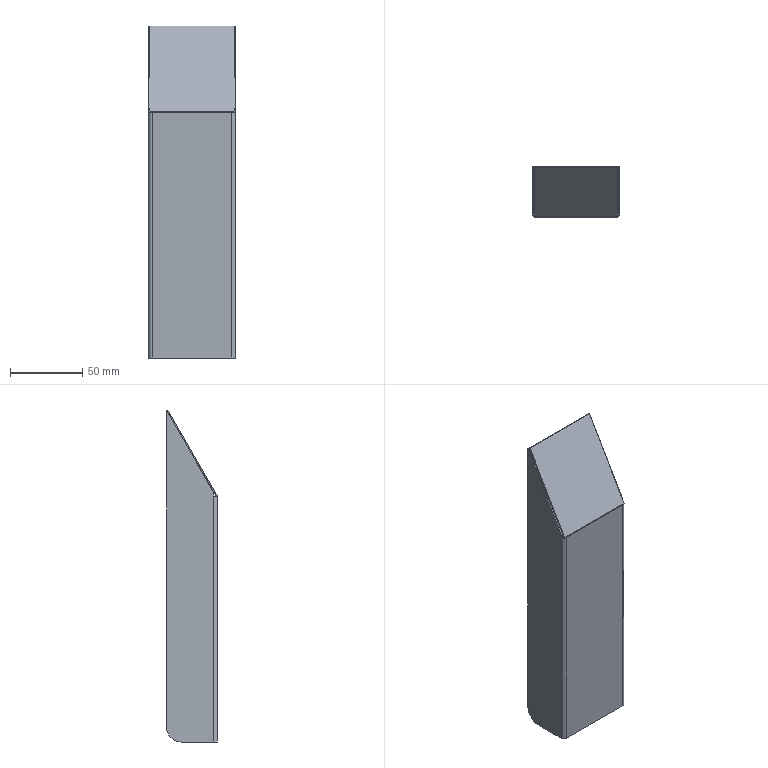Part | NX | 1 solid | 36 faces | box 60 x 35 x 229.016 mm | volume 27274 mm3 | plane 24 | cylinder 12 | commonest cylinder face diameters 4.5 x4 3.2 x2 5.2 x2 20 x2 0.8 x1 2.8 x1
STEP:
#1=CARTESIAN_POINT('',(2020.571,-112.446,-328.341));
#2=VERTEX_POINT('',#1);
#3=CARTESIAN_POINT('',(2020.571,-113.312,-327.841));
#4=VERTEX_POINT('',#3);
#5=CARTESIAN_POINT('',(2020.571,-112.446,-328.341));
#6=DIRECTION('',(0.,-0.866,0.5));
#7=VECTOR('',#6,1000.);
#8=LINE('',#5,#7);
#9=EDGE_CURVE('',#2,#4,#8,.T.);
#10=ORIENTED_EDGE('',*,*,#9,.T.);
#11=CARTESIAN_POINT('',(2020.571,-79.427,-269.151));
#12=VERTEX_POINT('',#11);
#13=CARTESIAN_POINT('',(2020.571,-171.235,-428.166));
#14=DIRECTION('',(0.,0.5,0.866));
#15=VECTOR('',#14,1000.);
#16=LINE('',#13,#15);
#17=EDGE_CURVE('',#4,#12,#16,.T.);
#18=ORIENTED_EDGE('',*,*,#17,.T.);
#19=CARTESIAN_POINT('',(2020.571,-78.561,-269.651));
#20=VERTEX_POINT('',#19);
#21=CARTESIAN_POINT('',(2020.571,-112.5,-250.056));
#22=DIRECTION('',(0.,0.866,-0.5));
#23=VECTOR('',#22,1000.);
#24=LINE('',#21,#23);
#25=EDGE_CURVE('',#12,#20,#24,.T.);
#26=ORIENTED_EDGE('',*,*,#25,.T.);
#27=CARTESIAN_POINT('',(2020.571,-170.08,-428.166));
#28=DIRECTION('',(0.,0.5,0.866));
#29=VECTOR('',#28,1000.);
#30=LINE('',#27,#29);
#31=EDGE_CURVE('',#2,#20,#30,.T.);
#32=ORIENTED_EDGE('',*,*,#31,.F.);
#33=EDGE_LOOP('',(#10,#18,#26,#32));
#34=FACE_BOUND('',#33,.T.);
#35=CARTESIAN_POINT('',(2020.571,-103.79,-313.348));
#36=DIRECTION('',(-1.,0.,0.));
#37=DIRECTION('',(0.,0.,1.));
#38=AXIS2_PLACEMENT_3D('',#35,#36,#37);
#39=PLANE('',#38);
#40=ADVANCED_FACE('',(#34),#39,.T.);
#41=CARTESIAN_POINT('',(2020.5,-88.5,-498.166));
#42=VERTEX_POINT('',#41);
#43=CARTESIAN_POINT('',(2019.5,-88.5,-498.166));
#44=VERTEX_POINT('',#43);
#45=CARTESIAN_POINT('',(1649.5,-88.5,-498.166));
#46=DIRECTION('',(-1.,0.,0.));
#47=VECTOR('',#46,1000.);
#48=LINE('',#45,#47);
#49=EDGE_CURVE('',#42,#44,#48,.T.);
#50=ORIENTED_EDGE('',*,*,#49,.F.);
#51=CARTESIAN_POINT('',(2020.5,-110.9,-498.166));
#52=VERTEX_POINT('',#51);
#53=CARTESIAN_POINT('',(2020.5,-112.5,-498.166));
#54=DIRECTION('',(0.,-1.,0.));
#55=VECTOR('',#54,1000.);
#56=LINE('',#53,#55);
#57=EDGE_CURVE('',#42,#52,#56,.T.);
#58=ORIENTED_EDGE('',*,*,#57,.T.);
#59=CARTESIAN_POINT('',(2022.1,-112.5,-498.166));
#60=VERTEX_POINT('',#59);
#61=CARTESIAN_POINT('',(2022.1,-110.9,-498.166));
#62=DIRECTION('',(0.,0.,1.));
#63=DIRECTION('',(-1.,0.,0.));
#64=AXIS2_PLACEMENT_3D('',#61,#62,#63);
#65=CIRCLE('',#64,1.6);
#66=EDGE_CURVE('',#52,#60,#65,.T.);
#67=ORIENTED_EDGE('',*,*,#66,.T.);
#68=CARTESIAN_POINT('',(2076.9,-112.5,-498.166));
#69=VERTEX_POINT('',#68);
#70=CARTESIAN_POINT('',(1649.5,-112.5,-498.166));
#71=DIRECTION('',(1.,0.,0.));
#72=VECTOR('',#71,1000.);
#73=LINE('',#70,#72);
#74=EDGE_CURVE('',#60,#69,#73,.T.);
#75=ORIENTED_EDGE('',*,*,#74,.T.);
#76=CARTESIAN_POINT('',(2078.5,-110.9,-498.166));
#77=VERTEX_POINT('',#76);
#78=CARTESIAN_POINT('',(2076.9,-110.9,-498.166));
#79=DIRECTION('',(0.,0.,-1.));
#80=DIRECTION('',(1.,0.,0.));
#81=AXIS2_PLACEMENT_3D('',#78,#79,#80);
#82=CIRCLE('',#81,1.6);
#83=EDGE_CURVE('',#77,#69,#82,.T.);
#84=ORIENTED_EDGE('',*,*,#83,.F.);
#85=CARTESIAN_POINT('',(2078.5,-88.5,-498.166));
#86=VERTEX_POINT('',#85);
#87=CARTESIAN_POINT('',(2078.5,-112.5,-498.166));
#88=DIRECTION('',(0.,1.,0.));
#89=VECTOR('',#88,1000.);
#90=LINE('',#87,#89);
#91=EDGE_CURVE('',#77,#86,#90,.T.);
#92=ORIENTED_EDGE('',*,*,#91,.T.);
#93=CARTESIAN_POINT('',(2079.5,-88.5,-498.166));
#94=VERTEX_POINT('',#93);
#95=CARTESIAN_POINT('',(1649.5,-88.5,-498.166));
#96=DIRECTION('',(-1.,0.,0.));
#97=VECTOR('',#96,1000.);
#98=LINE('',#95,#97);
#99=EDGE_CURVE('',#94,#86,#98,.T.);
#100=ORIENTED_EDGE('',*,*,#99,.F.);
#101=CARTESIAN_POINT('',(2079.5,-110.9,-498.166));
#102=VERTEX_POINT('',#101);
#103=CARTESIAN_POINT('',(2079.5,-112.5,-498.166));
#104=DIRECTION('',(0.,-1.,0.));
#105=VECTOR('',#104,1000.);
#106=LINE('',#103,#105);
#107=EDGE_CURVE('',#94,#102,#106,.T.);
#108=ORIENTED_EDGE('',*,*,#107,.T.);
#109=CARTESIAN_POINT('',(2076.9,-113.5,-498.166));
#110=VERTEX_POINT('',#109);
#111=CARTESIAN_POINT('',(2076.9,-110.9,-498.166));
#112=DIRECTION('',(0.,0.,-1.));
#113=DIRECTION('',(1.,0.,0.));
#114=AXIS2_PLACEMENT_3D('',#111,#112,#113);
#115=CIRCLE('',#114,2.6);
#116=EDGE_CURVE('',#102,#110,#115,.T.);
#117=ORIENTED_EDGE('',*,*,#116,.T.);
#118=CARTESIAN_POINT('',(2022.1,-113.5,-498.166));
#119=VERTEX_POINT('',#118);
#120=CARTESIAN_POINT('',(1649.5,-113.5,-498.166));
#121=DIRECTION('',(1.,0.,0.));
#122=VECTOR('',#121,1000.);
#123=LINE('',#120,#122);
#124=EDGE_CURVE('',#119,#110,#123,.T.);
#125=ORIENTED_EDGE('',*,*,#124,.F.);
#126=CARTESIAN_POINT('',(2019.5,-110.9,-498.166));
#127=VERTEX_POINT('',#126);
#128=CARTESIAN_POINT('',(2022.1,-110.9,-498.166));
#129=DIRECTION('',(0.,0.,1.));
#130=DIRECTION('',(-1.,0.,0.));
#131=AXIS2_PLACEMENT_3D('',#128,#129,#130);
#132=CIRCLE('',#131,2.6);
#133=EDGE_CURVE('',#127,#119,#132,.T.);
#134=ORIENTED_EDGE('',*,*,#133,.F.);
#135=CARTESIAN_POINT('',(2019.5,-112.5,-498.166));
#136=DIRECTION('',(0.,-1.,0.));
#137=VECTOR('',#136,1000.);
#138=LINE('',#135,#137);
#139=EDGE_CURVE('',#44,#127,#138,.T.);
#140=ORIENTED_EDGE('',*,*,#139,.F.);
#141=EDGE_LOOP('',(#50,#58,#67,#75,#84,#92,#100,#108,#117,#125,#134,#140));
#142=FACE_BOUND('',#141,.T.);
#143=CARTESIAN_POINT('',(2021.6,-170.4,-498.166));
#144=DIRECTION('',(0.,0.,-1.));
#145=DIRECTION('',(0.,-1.,0.));
#146=AXIS2_PLACEMENT_3D('',#143,#144,#145);
#147=PLANE('',#146);
#148=ADVANCED_FACE('',(#142),#147,.T.);
#149=CARTESIAN_POINT('',(2078.429,-113.312,-327.841));
#150=VERTEX_POINT('',#149);
#151=CARTESIAN_POINT('',(2078.429,-112.446,-328.341));
#152=VERTEX_POINT('',#151);
#153=CARTESIAN_POINT('',(2078.429,-112.446,-328.341));
#154=DIRECTION('',(0.,0.866,-0.5));
#155=VECTOR('',#154,1000.);
#156=LINE('',#153,#155);
#157=EDGE_CURVE('',#150,#152,#156,.T.);
#158=ORIENTED_EDGE('',*,*,#157,.T.);
#159=CARTESIAN_POINT('',(2078.429,-78.561,-269.651));
#160=VERTEX_POINT('',#159);
#161=CARTESIAN_POINT('',(2078.429,-170.08,-428.166));
#162=DIRECTION('',(0.,-0.5,-0.866));
#163=VECTOR('',#162,1000.);
#164=LINE('',#161,#163);
#165=EDGE_CURVE('',#160,#152,#164,.T.);
#166=ORIENTED_EDGE('',*,*,#165,.F.);
#167=CARTESIAN_POINT('',(2078.429,-79.427,-269.151));
#168=VERTEX_POINT('',#167);
#169=CARTESIAN_POINT('',(2078.429,-112.5,-250.056));
#170=DIRECTION('',(0.,-0.866,0.5));
#171=VECTOR('',#170,1000.);
#172=LINE('',#169,#171);
#173=EDGE_CURVE('',#160,#168,#172,.T.);
#174=ORIENTED_EDGE('',*,*,#173,.T.);
#175=CARTESIAN_POINT('',(2078.429,-171.235,-428.166));
#176=DIRECTION('',(0.,-0.5,-0.866));
#177=VECTOR('',#176,1000.);
#178=LINE('',#175,#177);
#179=EDGE_CURVE('',#168,#150,#178,.T.);
#180=ORIENTED_EDGE('',*,*,#179,.T.);
#181=EDGE_LOOP('',(#158,#166,#174,#180));
#182=FACE_BOUND('',#181,.T.);
#183=CARTESIAN_POINT('',(2078.429,-103.79,-313.348));
#184=DIRECTION('',(1.,0.,0.));
#185=DIRECTION('',(0.,1.,0.));
#186=AXIS2_PLACEMENT_3D('',#183,#184,#185);
#187=PLANE('',#186);
#188=ADVANCED_FACE('',(#182),#187,.T.);
#189=ORIENTED_EDGE('',*,*,#49,.T.);
#190=CARTESIAN_POINT('',(2019.5,-78.5,-488.166));
#191=VERTEX_POINT('',#190);
#192=CARTESIAN_POINT('',(2019.5,-88.5,-488.166));
#193=DIRECTION('',(-1.,0.,0.));
#194=DIRECTION('',(0.,0.,-1.));
#195=AXIS2_PLACEMENT_3D('',#192,#193,#194);
#196=CIRCLE('',#195,10.);
#197=EDGE_CURVE('',#191,#44,#196,.T.);
#198=ORIENTED_EDGE('',*,*,#197,.F.);
#199=CARTESIAN_POINT('',(2020.5,-78.5,-488.166));
#200=VERTEX_POINT('',#199);
#201=CARTESIAN_POINT('',(1649.5,-78.5,-488.166));
#202=DIRECTION('',(-1.,0.,0.));
#203=VECTOR('',#202,1000.);
#204=LINE('',#201,#203);
#205=EDGE_CURVE('',#200,#191,#204,.T.);
#206=ORIENTED_EDGE('',*,*,#205,.F.);
#207=CARTESIAN_POINT('',(2020.5,-88.5,-488.166));
#208=DIRECTION('',(-1.,0.,0.));
#209=DIRECTION('',(0.,0.,-1.));
#210=AXIS2_PLACEMENT_3D('',#207,#208,#209);
#211=CIRCLE('',#210,10.);
#212=EDGE_CURVE('',#200,#42,#211,.T.);
#213=ORIENTED_EDGE('',*,*,#212,.T.);
#214=EDGE_LOOP('',(#189,#198,#206,#213));
#215=FACE_BOUND('',#214,.T.);
#216=CARTESIAN_POINT('',(1649.5,-88.5,-488.166));
#217=DIRECTION('',(-1.,0.,0.));
#218=DIRECTION('',(0.,0.,-1.));
#219=AXIS2_PLACEMENT_3D('',#216,#217,#218);
#220=CYLINDRICAL_SURFACE('',#219,10.);
#221=ADVANCED_FACE('',(#215),#220,.T.);
#222=CARTESIAN_POINT('',(2079.5,-110.9,-328.541));
#223=VERTEX_POINT('',#222);
#224=CARTESIAN_POINT('',(2079.5,-110.9,-448.166));
#225=DIRECTION('',(0.,0.,-1.));
#226=VECTOR('',#225,1000.);
#227=LINE('',#224,#226);
#228=EDGE_CURVE('',#223,#102,#227,.T.);
#229=ORIENTED_EDGE('',*,*,#228,.T.);
#230=ORIENTED_EDGE('',*,*,#107,.F.);
#231=CARTESIAN_POINT('',(2079.5,-78.5,-488.166));
#232=VERTEX_POINT('',#231);
#233=CARTESIAN_POINT('',(2079.5,-88.5,-488.166));
#234=DIRECTION('',(-1.,0.,0.));
#235=DIRECTION('',(0.,0.,-1.));
#236=AXIS2_PLACEMENT_3D('',#233,#234,#235);
#237=CIRCLE('',#236,10.);
#238=EDGE_CURVE('',#232,#94,#237,.T.);
#239=ORIENTED_EDGE('',*,*,#238,.F.);
#240=CARTESIAN_POINT('',(2079.5,-78.5,-269.686));
#241=VERTEX_POINT('',#240);
#242=CARTESIAN_POINT('',(2079.5,-78.5,-428.166));
#243=DIRECTION('',(0.,0.,-1.));
#244=VECTOR('',#243,1000.);
#245=LINE('',#242,#244);
#246=EDGE_CURVE('',#241,#232,#245,.T.);
#247=ORIENTED_EDGE('',*,*,#246,.F.);
#248=CARTESIAN_POINT('',(2079.5,-110.9,-325.804));
#249=VERTEX_POINT('',#248);
#250=CARTESIAN_POINT('',(2079.5,-169.999,-428.166));
#251=DIRECTION('',(0.,0.5,0.866));
#252=VECTOR('',#251,1000.);
#253=LINE('',#250,#252);
#254=EDGE_CURVE('',#249,#241,#253,.T.);
#255=ORIENTED_EDGE('',*,*,#254,.F.);
#256=CARTESIAN_POINT('',(2079.5,-110.9,-428.166));
#257=DIRECTION('',(0.,0.,1.));
#258=VECTOR('',#257,1000.);
#259=LINE('',#256,#258);
#260=EDGE_CURVE('',#223,#249,#259,.T.);
#261=ORIENTED_EDGE('',*,*,#260,.F.);
#262=EDGE_LOOP('',(#229,#230,#239,#247,#255,#261));
#263=FACE_BOUND('',#262,.T.);
#264=CARTESIAN_POINT('',(2079.5,-86.551,-317.041));
#265=VERTEX_POINT('',#264);
#266=CARTESIAN_POINT('',(2079.5,-90.449,-319.291));
#267=VERTEX_POINT('',#266);
#268=CARTESIAN_POINT('',(2079.5,-88.5,-318.166));
#269=DIRECTION('',(-1.,0.,0.));
#270=DIRECTION('',(0.,-0.866,-0.5));
#271=AXIS2_PLACEMENT_3D('',#268,#269,#270);
#272=CIRCLE('',#271,2.25);
#273=EDGE_CURVE('',#265,#267,#272,.T.);
#274=ORIENTED_EDGE('',*,*,#273,.T.);
#275=CARTESIAN_POINT('',(2079.5,-88.5,-318.166));
#276=DIRECTION('',(-1.,0.,0.));
#277=DIRECTION('',(0.,-0.866,-0.5));
#278=AXIS2_PLACEMENT_3D('',#275,#276,#277);
#279=CIRCLE('',#278,2.25);
#280=EDGE_CURVE('',#267,#265,#279,.T.);
#281=ORIENTED_EDGE('',*,*,#280,.T.);
#282=EDGE_LOOP('',(#274,#281));
#283=FACE_BOUND('',#282,.T.);
#284=CARTESIAN_POINT('',(2079.5,-90.449,-364.291));
#285=VERTEX_POINT('',#284);
#286=CARTESIAN_POINT('',(2079.5,-86.551,-362.041));
#287=VERTEX_POINT('',#286);
#288=CARTESIAN_POINT('',(2079.5,-88.5,-363.166));
#289=DIRECTION('',(-1.,0.,0.));
#290=DIRECTION('',(0.,-0.866,-0.5));
#291=AXIS2_PLACEMENT_3D('',#288,#289,#290);
#292=CIRCLE('',#291,2.25);
#293=EDGE_CURVE('',#285,#287,#292,.T.);
#294=ORIENTED_EDGE('',*,*,#293,.T.);
#295=CARTESIAN_POINT('',(2079.5,-88.5,-363.166));
#296=DIRECTION('',(-1.,0.,0.));
#297=DIRECTION('',(0.,-0.866,-0.5));
#298=AXIS2_PLACEMENT_3D('',#295,#296,#297);
#299=CIRCLE('',#298,2.25);
#300=EDGE_CURVE('',#287,#285,#299,.T.);
#301=ORIENTED_EDGE('',*,*,#300,.T.);
#302=EDGE_LOOP('',(#294,#301));
#303=FACE_BOUND('',#302,.T.);
#304=CARTESIAN_POINT('',(2079.5,-541.4,-428.166));
#305=DIRECTION('',(-1.,0.,0.));
#306=DIRECTION('',(0.,0.,1.));
#307=AXIS2_PLACEMENT_3D('',#304,#305,#306);
#308=PLANE('',#307);
#309=ADVANCED_FACE('',(#263,#283,#303),#308,.F.);
#310=CARTESIAN_POINT('',(2022.1,-113.312,-327.841));
#311=VERTEX_POINT('',#310);
#312=CARTESIAN_POINT('',(2022.1,-113.5,-328.541));
#313=VERTEX_POINT('',#312);
#314=CARTESIAN_POINT('',(2022.1,-112.1,-328.541));
#315=DIRECTION('',(1.,0.,0.));
#316=DIRECTION('',(0.,-0.866,0.5));
#317=AXIS2_PLACEMENT_3D('',#314,#315,#316);
#318=CIRCLE('',#317,1.4);
#319=EDGE_CURVE('',#311,#313,#318,.T.);
#320=ORIENTED_EDGE('',*,*,#319,.T.);
#321=CARTESIAN_POINT('',(2076.9,-113.5,-328.541));
#322=VERTEX_POINT('',#321);
#323=CARTESIAN_POINT('',(1649.5,-113.5,-328.541));
#324=DIRECTION('',(-1.,0.,0.));
#325=VECTOR('',#324,1000.);
#326=LINE('',#323,#325);
#327=EDGE_CURVE('',#322,#313,#326,.T.);
#328=ORIENTED_EDGE('',*,*,#327,.F.);
#329=CARTESIAN_POINT('',(2076.9,-113.312,-327.841));
#330=VERTEX_POINT('',#329);
#331=CARTESIAN_POINT('',(2076.9,-112.1,-328.541));
#332=DIRECTION('',(-1.,0.,0.));
#333=DIRECTION('',(0.,-1.,0.));
#334=AXIS2_PLACEMENT_3D('',#331,#332,#333);
#335=CIRCLE('',#334,1.4);
#336=EDGE_CURVE('',#322,#330,#335,.T.);
#337=ORIENTED_EDGE('',*,*,#336,.T.);
#338=CARTESIAN_POINT('',(1649.5,-113.312,-327.841));
#339=DIRECTION('',(-1.,0.,0.));
#340=VECTOR('',#339,1000.);
#341=LINE('',#338,#340);
#342=EDGE_CURVE('',#330,#311,#341,.T.);
#343=ORIENTED_EDGE('',*,*,#342,.T.);
#344=EDGE_LOOP('',(#320,#328,#337,#343));
#345=FACE_BOUND('',#344,.T.);
#346=CARTESIAN_POINT('',(2076.9,-112.1,-328.541));
#347=DIRECTION('',(1.,0.,0.));
#348=DIRECTION('',(0.,0.,1.));
#349=AXIS2_PLACEMENT_3D('',#346,#347,#348);
#350=CYLINDRICAL_SURFACE('',#349,1.4);
#351=ADVANCED_FACE('',(#345),#350,.T.);
#352=CARTESIAN_POINT('',(1649.5,-113.312,-327.841));
#353=DIRECTION('',(1.,0.,0.));
#354=VECTOR('',#353,1000.);
#355=LINE('',#352,#354);
#356=EDGE_CURVE('',#4,#311,#355,.T.);
#357=ORIENTED_EDGE('',*,*,#356,.T.);
#358=ORIENTED_EDGE('',*,*,#342,.F.);
#359=CARTESIAN_POINT('',(1649.5,-113.312,-327.841));
#360=DIRECTION('',(1.,0.,0.));
#361=VECTOR('',#360,1000.);
#362=LINE('',#359,#361);
#363=EDGE_CURVE('',#330,#150,#362,.T.);
#364=ORIENTED_EDGE('',*,*,#363,.T.);
#365=ORIENTED_EDGE('',*,*,#179,.F.);
#366=CARTESIAN_POINT('',(1649.5,-79.427,-269.151));
#367=DIRECTION('',(1.,0.,0.));
#368=VECTOR('',#367,1000.);
#369=LINE('',#366,#368);
#370=EDGE_CURVE('',#12,#168,#369,.T.);
#371=ORIENTED_EDGE('',*,*,#370,.F.);
#372=ORIENTED_EDGE('',*,*,#17,.F.);
#373=EDGE_LOOP('',(#357,#358,#364,#365,#371,#372));
#374=FACE_BOUND('',#373,.T.);
#375=CARTESIAN_POINT('',(1649.5,-163.289,-414.403));
#376=DIRECTION('',(0.,0.866,-0.5));
#377=DIRECTION('',(-1.,0.,0.));
#378=AXIS2_PLACEMENT_3D('',#375,#376,#377);
#379=PLANE('',#378);
#380=ADVANCED_FACE('',(#374),#379,.F.);
#381=CARTESIAN_POINT('',(2076.9,-113.5,-428.166));
#382=DIRECTION('',(0.,0.,1.));
#383=VECTOR('',#382,1000.);
#384=LINE('',#381,#383);
#385=EDGE_CURVE('',#110,#322,#384,.T.);
#386=ORIENTED_EDGE('',*,*,#385,.F.);
#387=ORIENTED_EDGE('',*,*,#116,.F.);
#388=ORIENTED_EDGE('',*,*,#228,.F.);
#389=CARTESIAN_POINT('',(2076.9,-110.9,-328.541));
#390=DIRECTION('',(0.,0.,-1.));
#391=DIRECTION('',(1.,0.,0.));
#392=AXIS2_PLACEMENT_3D('',#389,#390,#391);
#393=CIRCLE('',#392,2.6);
#394=EDGE_CURVE('',#223,#322,#393,.T.);
#395=ORIENTED_EDGE('',*,*,#394,.T.);
#396=EDGE_LOOP('',(#386,#387,#388,#395));
#397=FACE_BOUND('',#396,.T.);
#398=CARTESIAN_POINT('',(2076.9,-110.9,-448.166));
#399=DIRECTION('',(0.,0.,-1.));
#400=DIRECTION('',(1.,0.,0.));
#401=AXIS2_PLACEMENT_3D('',#398,#399,#400);
#402=CYLINDRICAL_SURFACE('',#401,2.6);
#403=ADVANCED_FACE('',(#397),#402,.T.);
#404=CARTESIAN_POINT('',(2078.5,-86.551,-362.041));
#405=VERTEX_POINT('',#404);
#406=CARTESIAN_POINT('',(2078.5,-90.449,-364.291));
#407=VERTEX_POINT('',#406);
#408=CARTESIAN_POINT('',(2078.5,-88.5,-363.166));
#409=DIRECTION('',(-1.,0.,0.));
#410=DIRECTION('',(0.,-0.866,-0.5));
#411=AXIS2_PLACEMENT_3D('',#408,#409,#410);
#412=CIRCLE('',#411,2.25);
#413=EDGE_CURVE('',#405,#407,#412,.T.);
#414=ORIENTED_EDGE('',*,*,#413,.T.);
#415=CARTESIAN_POINT('',(2085.5,-90.449,-364.291));
#416=DIRECTION('',(-1.,0.,0.));
#417=VECTOR('',#416,1000.);
#418=LINE('',#415,#417);
#419=EDGE_CURVE('',#407,#285,#418,.F.);
#420=ORIENTED_EDGE('',*,*,#419,.T.);
#421=ORIENTED_EDGE('',*,*,#300,.F.);
#422=CARTESIAN_POINT('',(2085.5,-86.551,-362.041));
#423=DIRECTION('',(-1.,0.,0.));
#424=VECTOR('',#423,1000.);
#425=LINE('',#422,#424);
#426=EDGE_CURVE('',#405,#287,#425,.F.);
#427=ORIENTED_EDGE('',*,*,#426,.F.);
#428=EDGE_LOOP('',(#414,#420,#421,#427));
#429=FACE_BOUND('',#428,.T.);
#430=CARTESIAN_POINT('',(2085.5,-88.5,-363.166));
#431=DIRECTION('',(-1.,0.,0.));
#432=DIRECTION('',(0.,-0.866,-0.5));
#433=AXIS2_PLACEMENT_3D('',#430,#431,#432);
#434=CYLINDRICAL_SURFACE('',#433,2.25);
#435=ADVANCED_FACE('',(#429),#434,.F.);
#436=ORIENTED_EDGE('',*,*,#356,.F.);
#437=ORIENTED_EDGE('',*,*,#9,.F.);
#438=CARTESIAN_POINT('',(2022.1,-112.446,-328.341));
#439=VERTEX_POINT('',#438);
#440=CARTESIAN_POINT('',(1649.5,-112.446,-328.341));
#441=DIRECTION('',(-1.,0.,0.));
#442=VECTOR('',#441,1000.);
#443=LINE('',#440,#442);
#444=EDGE_CURVE('',#439,#2,#443,.T.);
#445=ORIENTED_EDGE('',*,*,#444,.F.);
#446=CARTESIAN_POINT('',(2022.1,-113.312,-327.841));
#447=DIRECTION('',(0.,0.866,-0.5));
#448=VECTOR('',#447,1000.);
#449=LINE('',#446,#448);
#450=EDGE_CURVE('',#311,#439,#449,.T.);
#451=ORIENTED_EDGE('',*,*,#450,.F.);
#452=EDGE_LOOP('',(#436,#437,#445,#451));
#453=FACE_BOUND('',#452,.T.);
#454=CARTESIAN_POINT('',(2019.,-113.312,-327.841));
#455=DIRECTION('',(0.,-0.5,-0.866));
#456=DIRECTION('',(0.,-0.866,0.5));
#457=AXIS2_PLACEMENT_3D('',#454,#455,#456);
#458=PLANE('',#457);
#459=ADVANCED_FACE('',(#453),#458,.T.);
#460=ORIENTED_EDGE('',*,*,#370,.T.);
#461=ORIENTED_EDGE('',*,*,#173,.F.);
#462=CARTESIAN_POINT('',(1649.5,-78.561,-269.651));
#463=DIRECTION('',(1.,0.,0.));
#464=VECTOR('',#463,1000.);
#465=LINE('',#462,#464);
#466=EDGE_CURVE('',#20,#160,#465,.T.);
#467=ORIENTED_EDGE('',*,*,#466,.F.);
#468=ORIENTED_EDGE('',*,*,#25,.F.);
#469=EDGE_LOOP('',(#460,#461,#467,#468));
#470=FACE_BOUND('',#469,.T.);
#471=CARTESIAN_POINT('',(2079.5,-79.427,-269.151));
#472=DIRECTION('',(0.,0.5,0.866));
#473=DIRECTION('',(1.,0.,0.));
#474=AXIS2_PLACEMENT_3D('',#471,#472,#473);
#475=PLANE('',#474);
#476=ADVANCED_FACE('',(#470),#475,.T.);
#477=CARTESIAN_POINT('',(2078.5,-110.9,-325.804));
#478=VERTEX_POINT('',#477);
#479=CARTESIAN_POINT('',(2078.5,-78.5,-269.686));
#480=VERTEX_POINT('',#479);
#481=CARTESIAN_POINT('',(2078.5,-169.999,-428.166));
#482=DIRECTION('',(0.,0.5,0.866));
#483=VECTOR('',#482,1000.);
#484=LINE('',#481,#483);
#485=EDGE_CURVE('',#478,#480,#484,.T.);
#486=ORIENTED_EDGE('',*,*,#485,.T.);
#487=CARTESIAN_POINT('',(2078.5,-78.5,-488.166));
#488=VERTEX_POINT('',#487);
#489=CARTESIAN_POINT('',(2078.5,-78.5,-428.166));
#490=DIRECTION('',(0.,0.,1.));
#491=VECTOR('',#490,1000.);
#492=LINE('',#489,#491);
#493=EDGE_CURVE('',#488,#480,#492,.T.);
#494=ORIENTED_EDGE('',*,*,#493,.F.);
#495=CARTESIAN_POINT('',(2078.5,-88.5,-488.166));
#496=DIRECTION('',(-1.,0.,0.));
#497=DIRECTION('',(0.,0.,-1.));
#498=AXIS2_PLACEMENT_3D('',#495,#496,#497);
#499=CIRCLE('',#498,10.);
#500=EDGE_CURVE('',#488,#86,#499,.T.);
#501=ORIENTED_EDGE('',*,*,#500,.T.);
#502=ORIENTED_EDGE('',*,*,#91,.F.);
#503=CARTESIAN_POINT('',(2078.5,-110.9,-328.541));
#504=VERTEX_POINT('',#503);
#505=CARTESIAN_POINT('',(2078.5,-110.9,-448.166));
#506=DIRECTION('',(0.,0.,-1.));
#507=VECTOR('',#506,1000.);
#508=LINE('',#505,#507);
#509=EDGE_CURVE('',#504,#77,#508,.T.);
#510=ORIENTED_EDGE('',*,*,#509,.F.);
#511=CARTESIAN_POINT('',(2078.5,-110.9,-428.166));
#512=DIRECTION('',(0.,0.,-1.));
#513=VECTOR('',#512,1000.);
#514=LINE('',#511,#513);
#515=EDGE_CURVE('',#478,#504,#514,.T.);
#516=ORIENTED_EDGE('',*,*,#515,.F.);
#517=EDGE_LOOP('',(#486,#494,#501,#502,#510,#516));
#518=FACE_BOUND('',#517,.T.);
#519=ORIENTED_EDGE('',*,*,#413,.F.);
#520=CARTESIAN_POINT('',(2078.5,-88.5,-363.166));
#521=DIRECTION('',(-1.,0.,0.));
#522=DIRECTION('',(0.,-0.866,-0.5));
#523=AXIS2_PLACEMENT_3D('',#520,#521,#522);
#524=CIRCLE('',#523,2.25);
#525=EDGE_CURVE('',#407,#405,#524,.T.);
#526=ORIENTED_EDGE('',*,*,#525,.F.);
#527=EDGE_LOOP('',(#519,#526));
#528=FACE_BOUND('',#527,.T.);
#529=CARTESIAN_POINT('',(2078.5,-90.449,-319.291));
#530=VERTEX_POINT('',#529);
#531=CARTESIAN_POINT('',(2078.5,-86.551,-317.041));
#532=VERTEX_POINT('',#531);
#533=CARTESIAN_POINT('',(2078.5,-88.5,-318.166));
#534=DIRECTION('',(-1.,0.,0.));
#535=DIRECTION('',(0.,-0.866,-0.5));
#536=AXIS2_PLACEMENT_3D('',#533,#534,#535);
#537=CIRCLE('',#536,2.25);
#538=EDGE_CURVE('',#530,#532,#537,.T.);
#539=ORIENTED_EDGE('',*,*,#538,.F.);
#540=CARTESIAN_POINT('',(2078.5,-88.5,-318.166));
#541=DIRECTION('',(-1.,0.,0.));
#542=DIRECTION('',(0.,-0.866,-0.5));
#543=AXIS2_PLACEMENT_3D('',#540,#541,#542);
#544=CIRCLE('',#543,2.25);
#545=EDGE_CURVE('',#532,#530,#544,.T.);
#546=ORIENTED_EDGE('',*,*,#545,.F.);
#547=EDGE_LOOP('',(#539,#546));
#548=FACE_BOUND('',#547,.T.);
#549=CARTESIAN_POINT('',(2078.5,-111.4,-328.541));
#550=DIRECTION('',(1.,0.,0.));
#551=DIRECTION('',(0.,1.,0.));
#552=AXIS2_PLACEMENT_3D('',#549,#550,#551);
#553=PLANE('',#552);
#554=ADVANCED_FACE('',(#518,#528,#548),#553,.F.);
#555=CARTESIAN_POINT('',(1649.5,-78.5,-488.166));
#556=DIRECTION('',(-1.,0.,0.));
#557=VECTOR('',#556,1000.);
#558=LINE('',#555,#557);
#559=EDGE_CURVE('',#232,#488,#558,.T.);
#560=ORIENTED_EDGE('',*,*,#559,.T.);
#561=ORIENTED_EDGE('',*,*,#493,.T.);
#562=CARTESIAN_POINT('',(1649.5,-78.5,-269.686));
#563=DIRECTION('',(-1.,0.,0.));
#564=VECTOR('',#563,1000.);
#565=LINE('',#562,#564);
#566=EDGE_CURVE('',#241,#480,#565,.T.);
#567=ORIENTED_EDGE('',*,*,#566,.F.);
#568=ORIENTED_EDGE('',*,*,#246,.T.);
#569=EDGE_LOOP('',(#560,#561,#567,#568));
#570=FACE_BOUND('',#569,.T.);
#571=CARTESIAN_POINT('',(2079.5,-78.5,-448.166));
#572=DIRECTION('',(0.,1.,0.));
#573=DIRECTION('',(1.,0.,0.));
#574=AXIS2_PLACEMENT_3D('',#571,#572,#573);
#575=PLANE('',#574);
#576=ADVANCED_FACE('',(#570),#575,.T.);
#577=ORIENTED_EDGE('',*,*,#254,.T.);
#578=ORIENTED_EDGE('',*,*,#566,.T.);
#579=ORIENTED_EDGE('',*,*,#485,.F.);
#580=CARTESIAN_POINT('',(2079.5,-110.9,-325.804));
#581=DIRECTION('',(-1.,0.,0.));
#582=VECTOR('',#581,1000.);
#583=LINE('',#580,#582);
#584=EDGE_CURVE('',#249,#478,#583,.T.);
#585=ORIENTED_EDGE('',*,*,#584,.F.);
#586=EDGE_LOOP('',(#577,#578,#579,#585));
#587=FACE_BOUND('',#586,.T.);
#588=CARTESIAN_POINT('',(2079.5,-83.5,-278.346));
#589=DIRECTION('',(0.,-0.866,0.5));
#590=DIRECTION('',(-1.,0.,0.));
#591=AXIS2_PLACEMENT_3D('',#588,#589,#590);
#592=PLANE('',#591);
#593=ADVANCED_FACE('',(#587),#592,.T.);
#594=ORIENTED_EDGE('',*,*,#260,.T.);
#595=ORIENTED_EDGE('',*,*,#584,.T.);
#596=ORIENTED_EDGE('',*,*,#515,.T.);
#597=CARTESIAN_POINT('',(2079.5,-110.9,-328.541));
#598=DIRECTION('',(-1.,0.,0.));
#599=VECTOR('',#598,1000.);
#600=LINE('',#597,#599);
#601=EDGE_CURVE('',#223,#504,#600,.T.);
#602=ORIENTED_EDGE('',*,*,#601,.F.);
#603=EDGE_LOOP('',(#594,#595,#596,#602));
#604=FACE_BOUND('',#603,.T.);
#605=CARTESIAN_POINT('',(2079.5,-110.9,-328.214));
#606=DIRECTION('',(0.,-1.,0.));
#607=DIRECTION('',(-1.,0.,0.));
#608=AXIS2_PLACEMENT_3D('',#605,#606,#607);
#609=PLANE('',#608);
#610=ADVANCED_FACE('',(#604),#609,.T.);
#611=CARTESIAN_POINT('',(2076.9,-112.5,-328.541));
#612=VERTEX_POINT('',#611);
#613=CARTESIAN_POINT('',(2076.9,-112.5,-428.166));
#614=DIRECTION('',(0.,0.,-1.));
#615=VECTOR('',#614,1000.);
#616=LINE('',#613,#615);
#617=EDGE_CURVE('',#612,#69,#616,.T.);
#618=ORIENTED_EDGE('',*,*,#617,.T.);
#619=ORIENTED_EDGE('',*,*,#74,.F.);
#620=CARTESIAN_POINT('',(2022.1,-112.5,-328.541));
#621=VERTEX_POINT('',#620);
#622=CARTESIAN_POINT('',(2022.1,-112.5,-428.166));
#623=DIRECTION('',(0.,0.,1.));
#624=VECTOR('',#623,1000.);
#625=LINE('',#622,#624);
#626=EDGE_CURVE('',#60,#621,#625,.T.);
#627=ORIENTED_EDGE('',*,*,#626,.T.);
#628=CARTESIAN_POINT('',(1649.5,-112.5,-328.541));
#629=DIRECTION('',(-1.,0.,0.));
#630=VECTOR('',#629,1000.);
#631=LINE('',#628,#630);
#632=EDGE_CURVE('',#612,#621,#631,.T.);
#633=ORIENTED_EDGE('',*,*,#632,.F.);
#634=EDGE_LOOP('',(#618,#619,#627,#633));
#635=FACE_BOUND('',#634,.T.);
#636=CARTESIAN_POINT('',(2079.5,-112.5,-328.541));
#637=DIRECTION('',(0.,-1.,0.));
#638=DIRECTION('',(0.,0.,-1.));
#639=AXIS2_PLACEMENT_3D('',#636,#637,#638);
#640=PLANE('',#639);
#641=ADVANCED_FACE('',(#635),#640,.F.);
#642=ORIENTED_EDGE('',*,*,#509,.T.);
#643=ORIENTED_EDGE('',*,*,#83,.T.);
#644=ORIENTED_EDGE('',*,*,#617,.F.);
#645=CARTESIAN_POINT('',(2076.9,-110.9,-328.541));
#646=DIRECTION('',(0.,0.,1.));
#647=DIRECTION('',(0.,-1.,0.));
#648=AXIS2_PLACEMENT_3D('',#645,#646,#647);
#649=CIRCLE('',#648,1.6);
#650=EDGE_CURVE('',#612,#504,#649,.T.);
#651=ORIENTED_EDGE('',*,*,#650,.T.);
#652=EDGE_LOOP('',(#642,#643,#644,#651));
#653=FACE_BOUND('',#652,.T.);
#654=CARTESIAN_POINT('',(2076.9,-110.9,-448.166));
#655=DIRECTION('',(0.,0.,-1.));
#656=DIRECTION('',(1.,0.,0.));
#657=AXIS2_PLACEMENT_3D('',#654,#655,#656);
#658=CYLINDRICAL_SURFACE('',#657,1.6);
#659=ADVANCED_FACE('',(#653),#658,.F.);
#660=ORIENTED_EDGE('',*,*,#626,.F.);
#661=ORIENTED_EDGE('',*,*,#66,.F.);
#662=CARTESIAN_POINT('',(2020.5,-110.9,-328.541));
#663=VERTEX_POINT('',#662);
#664=CARTESIAN_POINT('',(2020.5,-110.9,-328.541));
#665=DIRECTION('',(0.,0.,1.));
#666=VECTOR('',#665,1000.);
#667=LINE('',#664,#666);
#668=EDGE_CURVE('',#52,#663,#667,.T.);
#669=ORIENTED_EDGE('',*,*,#668,.T.);
#670=CARTESIAN_POINT('',(2022.1,-110.9,-328.541));
#671=DIRECTION('',(0.,0.,-1.));
#672=DIRECTION('',(0.,-1.,0.));
#673=AXIS2_PLACEMENT_3D('',#670,#671,#672);
#674=CIRCLE('',#673,1.6);
#675=EDGE_CURVE('',#621,#663,#674,.T.);
#676=ORIENTED_EDGE('',*,*,#675,.F.);
#677=EDGE_LOOP('',(#660,#661,#669,#676));
#678=FACE_BOUND('',#677,.T.);
#679=CARTESIAN_POINT('',(2022.1,-110.9,-328.541));
#680=DIRECTION('',(0.,0.,1.));
#681=DIRECTION('',(-1.,0.,0.));
#682=AXIS2_PLACEMENT_3D('',#679,#680,#681);
#683=CYLINDRICAL_SURFACE('',#682,1.6);
#684=ADVANCED_FACE('',(#678),#683,.F.);
#685=ORIENTED_EDGE('',*,*,#668,.F.);
#686=ORIENTED_EDGE('',*,*,#57,.F.);
#687=ORIENTED_EDGE('',*,*,#212,.F.);
#688=CARTESIAN_POINT('',(2020.5,-78.5,-269.686));
#689=VERTEX_POINT('',#688);
#690=CARTESIAN_POINT('',(2020.5,-78.5,-428.166));
#691=DIRECTION('',(0.,0.,-1.));
#692=VECTOR('',#691,1000.);
#693=LINE('',#690,#692);
#694=EDGE_CURVE('',#689,#200,#693,.T.);
#695=ORIENTED_EDGE('',*,*,#694,.F.);
#696=CARTESIAN_POINT('',(2020.5,-110.9,-325.804));
#697=VERTEX_POINT('',#696);
#698=CARTESIAN_POINT('',(2020.5,-169.999,-428.166));
#699=DIRECTION('',(0.,-0.5,-0.866));
#700=VECTOR('',#699,1000.);
#701=LINE('',#698,#700);
#702=EDGE_CURVE('',#689,#697,#701,.T.);
#703=ORIENTED_EDGE('',*,*,#702,.T.);
#704=CARTESIAN_POINT('',(2020.5,-110.9,-428.166));
#705=DIRECTION('',(0.,0.,1.));
#706=VECTOR('',#705,1000.);
#707=LINE('',#704,#706);
#708=EDGE_CURVE('',#663,#697,#707,.T.);
#709=ORIENTED_EDGE('',*,*,#708,.F.);
#710=EDGE_LOOP('',(#685,#686,#687,#695,#703,#709));
#711=FACE_BOUND('',#710,.T.);
#712=CARTESIAN_POINT('',(2020.5,-171.4,-328.541));
#713=DIRECTION('',(-1.,0.,0.));
#714=DIRECTION('',(0.,0.,1.));
#715=AXIS2_PLACEMENT_3D('',#712,#713,#714);
#716=PLANE('',#715);
#717=ADVANCED_FACE('',(#711),#716,.F.);
#718=ORIENTED_EDGE('',*,*,#273,.F.);
#719=CARTESIAN_POINT('',(2085.5,-86.551,-317.041));
#720=DIRECTION('',(-1.,0.,0.));
#721=VECTOR('',#720,1000.);
#722=LINE('',#719,#721);
#723=EDGE_CURVE('',#265,#532,#722,.T.);
#724=ORIENTED_EDGE('',*,*,#723,.T.);
#725=ORIENTED_EDGE('',*,*,#545,.T.);
#726=CARTESIAN_POINT('',(2085.5,-90.449,-319.291));
#727=DIRECTION('',(-1.,0.,0.));
#728=VECTOR('',#727,1000.);
#729=LINE('',#726,#728);
#730=EDGE_CURVE('',#267,#530,#729,.T.);
#731=ORIENTED_EDGE('',*,*,#730,.F.);
#732=EDGE_LOOP('',(#718,#724,#725,#731));
#733=FACE_BOUND('',#732,.T.);
#734=CARTESIAN_POINT('',(2085.5,-88.5,-318.166));
#735=DIRECTION('',(-1.,0.,0.));
#736=DIRECTION('',(0.,-0.866,-0.5));
#737=AXIS2_PLACEMENT_3D('',#734,#735,#736);
#738=CYLINDRICAL_SURFACE('',#737,2.25);
#739=ADVANCED_FACE('',(#733),#738,.F.);
#740=ORIENTED_EDGE('',*,*,#559,.F.);
#741=ORIENTED_EDGE('',*,*,#238,.T.);
#742=ORIENTED_EDGE('',*,*,#99,.T.);
#743=ORIENTED_EDGE('',*,*,#500,.F.);
#744=EDGE_LOOP('',(#740,#741,#742,#743));
#745=FACE_BOUND('',#744,.T.);
#746=CARTESIAN_POINT('',(1649.5,-88.5,-488.166));
#747=DIRECTION('',(-1.,0.,0.));
#748=DIRECTION('',(0.,0.,-1.));
#749=AXIS2_PLACEMENT_3D('',#746,#747,#748);
#750=CYLINDRICAL_SURFACE('',#749,10.);
#751=ADVANCED_FACE('',(#745),#750,.T.);
#752=ORIENTED_EDGE('',*,*,#319,.F.);
#753=ORIENTED_EDGE('',*,*,#450,.T.);
#754=CARTESIAN_POINT('',(2022.1,-112.1,-328.541));
#755=DIRECTION('',(-1.,0.,0.));
#756=DIRECTION('',(0.,-1.,0.));
#757=AXIS2_PLACEMENT_3D('',#754,#755,#756);
#758=CIRCLE('',#757,0.4);
#759=EDGE_CURVE('',#621,#439,#758,.T.);
#760=ORIENTED_EDGE('',*,*,#759,.F.);
#761=CARTESIAN_POINT('',(2022.1,-113.5,-328.541));
#762=DIRECTION('',(0.,1.,0.));
#763=VECTOR('',#762,1000.);
#764=LINE('',#761,#763);
#765=EDGE_CURVE('',#313,#621,#764,.T.);
#766=ORIENTED_EDGE('',*,*,#765,.F.);
#767=EDGE_LOOP('',(#752,#753,#760,#766));
#768=FACE_BOUND('',#767,.T.);
#769=CARTESIAN_POINT('',(2022.1,-112.1,-328.541));
#770=DIRECTION('',(1.,0.,0.));
#771=DIRECTION('',(0.,1.,0.));
#772=AXIS2_PLACEMENT_3D('',#769,#770,#771);
#773=PLANE('',#772);
#774=ADVANCED_FACE('',(#768),#773,.F.);
#775=CARTESIAN_POINT('',(2019.5,-78.5,-269.686));
#776=VERTEX_POINT('',#775);
#777=CARTESIAN_POINT('',(2019.5,-78.5,-428.166));
#778=DIRECTION('',(0.,0.,-1.));
#779=VECTOR('',#778,1000.);
#780=LINE('',#777,#779);
#781=EDGE_CURVE('',#776,#191,#780,.T.);
#782=ORIENTED_EDGE('',*,*,#781,.F.);
#783=CARTESIAN_POINT('',(1649.5,-78.5,-269.686));
#784=DIRECTION('',(-1.,0.,0.));
#785=VECTOR('',#784,1000.);
#786=LINE('',#783,#785);
#787=EDGE_CURVE('',#689,#776,#786,.T.);
#788=ORIENTED_EDGE('',*,*,#787,.F.);
#789=ORIENTED_EDGE('',*,*,#694,.T.);
#790=ORIENTED_EDGE('',*,*,#205,.T.);
#791=EDGE_LOOP('',(#782,#788,#789,#790));
#792=FACE_BOUND('',#791,.T.);
#793=CARTESIAN_POINT('',(2019.5,-78.5,-278.346));
#794=DIRECTION('',(0.,1.,0.));
#795=DIRECTION('',(1.,0.,0.));
#796=AXIS2_PLACEMENT_3D('',#793,#794,#795);
#797=PLANE('',#796);
#798=ADVANCED_FACE('',(#792),#797,.T.);
#799=CARTESIAN_POINT('',(2019.5,-110.9,-328.541));
#800=VERTEX_POINT('',#799);
#801=CARTESIAN_POINT('',(2022.1,-110.9,-328.541));
#802=DIRECTION('',(0.,0.,-1.));
#803=DIRECTION('',(0.,-1.,0.));
#804=AXIS2_PLACEMENT_3D('',#801,#802,#803);
#805=CIRCLE('',#804,2.6);
#806=EDGE_CURVE('',#313,#800,#805,.T.);
#807=ORIENTED_EDGE('',*,*,#806,.T.);
#808=CARTESIAN_POINT('',(2019.5,-110.9,-328.541));
#809=DIRECTION('',(0.,0.,1.));
#810=VECTOR('',#809,1000.);
#811=LINE('',#808,#810);
#812=EDGE_CURVE('',#127,#800,#811,.T.);
#813=ORIENTED_EDGE('',*,*,#812,.F.);
#814=ORIENTED_EDGE('',*,*,#133,.T.);
#815=CARTESIAN_POINT('',(2022.1,-113.5,-428.166));
#816=DIRECTION('',(0.,0.,1.));
#817=VECTOR('',#816,1000.);
#818=LINE('',#815,#817);
#819=EDGE_CURVE('',#119,#313,#818,.T.);
#820=ORIENTED_EDGE('',*,*,#819,.T.);
#821=EDGE_LOOP('',(#807,#813,#814,#820));
#822=FACE_BOUND('',#821,.T.);
#823=CARTESIAN_POINT('',(2022.1,-110.9,-328.541));
#824=DIRECTION('',(0.,0.,1.));
#825=DIRECTION('',(-1.,0.,0.));
#826=AXIS2_PLACEMENT_3D('',#823,#824,#825);
#827=CYLINDRICAL_SURFACE('',#826,2.6);
#828=ADVANCED_FACE('',(#822),#827,.T.);
#829=CARTESIAN_POINT('',(2019.5,-110.9,-325.804));
#830=VERTEX_POINT('',#829);
#831=CARTESIAN_POINT('',(2019.5,-110.9,-325.804));
#832=DIRECTION('',(-1.,0.,0.));
#833=VECTOR('',#832,1000.);
#834=LINE('',#831,#833);
#835=EDGE_CURVE('',#697,#830,#834,.T.);
#836=ORIENTED_EDGE('',*,*,#835,.F.);
#837=ORIENTED_EDGE('',*,*,#702,.F.);
#838=ORIENTED_EDGE('',*,*,#787,.T.);
#839=CARTESIAN_POINT('',(2019.5,-169.999,-428.166));
#840=DIRECTION('',(0.,-0.5,-0.866));
#841=VECTOR('',#840,1000.);
#842=LINE('',#839,#841);
#843=EDGE_CURVE('',#776,#830,#842,.T.);
#844=ORIENTED_EDGE('',*,*,#843,.T.);
#845=EDGE_LOOP('',(#836,#837,#838,#844));
#846=FACE_BOUND('',#845,.T.);
#847=CARTESIAN_POINT('',(2019.5,-111.4,-326.67));
#848=DIRECTION('',(0.,-0.866,0.5));
#849=DIRECTION('',(-1.,0.,0.));
#850=AXIS2_PLACEMENT_3D('',#847,#848,#849);
#851=PLANE('',#850);
#852=ADVANCED_FACE('',(#846),#851,.T.);
#853=ORIENTED_EDGE('',*,*,#806,.F.);
#854=ORIENTED_EDGE('',*,*,#765,.T.);
#855=ORIENTED_EDGE('',*,*,#675,.T.);
#856=CARTESIAN_POINT('',(2019.5,-110.9,-328.541));
#857=DIRECTION('',(1.,0.,0.));
#858=VECTOR('',#857,1000.);
#859=LINE('',#856,#858);
#860=EDGE_CURVE('',#800,#663,#859,.T.);
#861=ORIENTED_EDGE('',*,*,#860,.F.);
#862=EDGE_LOOP('',(#853,#854,#855,#861));
#863=FACE_BOUND('',#862,.T.);
#864=CARTESIAN_POINT('',(2022.1,-110.9,-328.541));
#865=DIRECTION('',(0.,0.,-1.));
#866=DIRECTION('',(0.,-1.,0.));
#867=AXIS2_PLACEMENT_3D('',#864,#865,#866);
#868=PLANE('',#867);
#869=ADVANCED_FACE('',(#863),#868,.F.);
#870=ORIENTED_EDGE('',*,*,#819,.F.);
#871=ORIENTED_EDGE('',*,*,#124,.T.);
#872=ORIENTED_EDGE('',*,*,#385,.T.);
#873=ORIENTED_EDGE('',*,*,#327,.T.);
#874=EDGE_LOOP('',(#870,#871,#872,#873));
#875=FACE_BOUND('',#874,.T.);
#876=CARTESIAN_POINT('',(2019.5,-113.5,-448.166));
#877=DIRECTION('',(0.,-1.,0.));
#878=DIRECTION('',(0.,0.,-1.));
#879=AXIS2_PLACEMENT_3D('',#876,#877,#878);
#880=PLANE('',#879);
#881=ADVANCED_FACE('',(#875),#880,.T.);
#882=ORIENTED_EDGE('',*,*,#812,.T.);
#883=CARTESIAN_POINT('',(2019.5,-110.9,-428.166));
#884=DIRECTION('',(0.,0.,1.));
#885=VECTOR('',#884,1000.);
#886=LINE('',#883,#885);
#887=EDGE_CURVE('',#800,#830,#886,.T.);
#888=ORIENTED_EDGE('',*,*,#887,.T.);
#889=ORIENTED_EDGE('',*,*,#843,.F.);
#890=ORIENTED_EDGE('',*,*,#781,.T.);
#891=ORIENTED_EDGE('',*,*,#197,.T.);
#892=ORIENTED_EDGE('',*,*,#139,.T.);
#893=EDGE_LOOP('',(#882,#888,#889,#890,#891,#892));
#894=FACE_BOUND('',#893,.T.);
#895=CARTESIAN_POINT('',(2019.5,-111.4,-448.166));
#896=DIRECTION('',(-1.,0.,0.));
#897=DIRECTION('',(0.,0.,1.));
#898=AXIS2_PLACEMENT_3D('',#895,#896,#897);
#899=PLANE('',#898);
#900=ADVANCED_FACE('',(#894),#899,.T.);
#901=ORIENTED_EDGE('',*,*,#336,.F.);
#902=CARTESIAN_POINT('',(2076.9,-113.5,-328.541));
#903=DIRECTION('',(0.,1.,0.));
#904=VECTOR('',#903,1000.);
#905=LINE('',#902,#904);
#906=EDGE_CURVE('',#322,#612,#905,.T.);
#907=ORIENTED_EDGE('',*,*,#906,.T.);
#908=CARTESIAN_POINT('',(2076.9,-112.446,-328.341));
#909=VERTEX_POINT('',#908);
#910=CARTESIAN_POINT('',(2076.9,-112.1,-328.541));
#911=DIRECTION('',(1.,0.,0.));
#912=DIRECTION('',(0.,-0.866,0.5));
#913=AXIS2_PLACEMENT_3D('',#910,#911,#912);
#914=CIRCLE('',#913,0.4);
#915=EDGE_CURVE('',#909,#612,#914,.T.);
#916=ORIENTED_EDGE('',*,*,#915,.F.);
#917=CARTESIAN_POINT('',(2076.9,-113.312,-327.841));
#918=DIRECTION('',(0.,0.866,-0.5));
#919=VECTOR('',#918,1000.);
#920=LINE('',#917,#919);
#921=EDGE_CURVE('',#330,#909,#920,.T.);
#922=ORIENTED_EDGE('',*,*,#921,.F.);
#923=EDGE_LOOP('',(#901,#907,#916,#922));
#924=FACE_BOUND('',#923,.T.);
#925=CARTESIAN_POINT('',(2076.9,-112.1,-328.541));
#926=DIRECTION('',(-1.,0.,0.));
#927=DIRECTION('',(0.,0.,1.));
#928=AXIS2_PLACEMENT_3D('',#925,#926,#927);
#929=PLANE('',#928);
#930=ADVANCED_FACE('',(#924),#929,.F.);
#931=ORIENTED_EDGE('',*,*,#759,.T.);
#932=CARTESIAN_POINT('',(1649.5,-112.446,-328.341));
#933=DIRECTION('',(-1.,0.,0.));
#934=VECTOR('',#933,1000.);
#935=LINE('',#932,#934);
#936=EDGE_CURVE('',#909,#439,#935,.T.);
#937=ORIENTED_EDGE('',*,*,#936,.F.);
#938=ORIENTED_EDGE('',*,*,#915,.T.);
#939=ORIENTED_EDGE('',*,*,#632,.T.);
#940=EDGE_LOOP('',(#931,#937,#938,#939));
#941=FACE_BOUND('',#940,.T.);
#942=CARTESIAN_POINT('',(2076.9,-112.1,-328.541));
#943=DIRECTION('',(1.,0.,0.));
#944=DIRECTION('',(0.,0.,1.));
#945=AXIS2_PLACEMENT_3D('',#942,#943,#944);
#946=CYLINDRICAL_SURFACE('',#945,0.4);
#947=ADVANCED_FACE('',(#941),#946,.F.);
#948=ORIENTED_EDGE('',*,*,#31,.T.);
#949=ORIENTED_EDGE('',*,*,#466,.T.);
#950=ORIENTED_EDGE('',*,*,#165,.T.);
#951=CARTESIAN_POINT('',(1649.5,-112.446,-328.341));
#952=DIRECTION('',(-1.,0.,0.));
#953=VECTOR('',#952,1000.);
#954=LINE('',#951,#953);
#955=EDGE_CURVE('',#152,#909,#954,.T.);
#956=ORIENTED_EDGE('',*,*,#955,.T.);
#957=ORIENTED_EDGE('',*,*,#936,.T.);
#958=ORIENTED_EDGE('',*,*,#444,.T.);
#959=EDGE_LOOP('',(#948,#949,#950,#956,#957,#958));
#960=FACE_BOUND('',#959,.T.);
#961=CARTESIAN_POINT('',(1649.5,-162.423,-414.903));
#962=DIRECTION('',(0.,0.866,-0.5));
#963=DIRECTION('',(-1.,0.,0.));
#964=AXIS2_PLACEMENT_3D('',#961,#962,#963);
#965=PLANE('',#964);
#966=ADVANCED_FACE('',(#960),#965,.T.);
#967=ORIENTED_EDGE('',*,*,#394,.F.);
#968=ORIENTED_EDGE('',*,*,#601,.T.);
#969=ORIENTED_EDGE('',*,*,#650,.F.);
#970=ORIENTED_EDGE('',*,*,#906,.F.);
#971=EDGE_LOOP('',(#967,#968,#969,#970));
#972=FACE_BOUND('',#971,.T.);
#973=CARTESIAN_POINT('',(2076.9,-110.9,-328.541));
#974=DIRECTION('',(0.,0.,-1.));
#975=DIRECTION('',(0.,-1.,0.));
#976=AXIS2_PLACEMENT_3D('',#973,#974,#975);
#977=PLANE('',#976);
#978=ADVANCED_FACE('',(#972),#977,.F.);
#979=ORIENTED_EDGE('',*,*,#363,.F.);
#980=ORIENTED_EDGE('',*,*,#921,.T.);
#981=ORIENTED_EDGE('',*,*,#955,.F.);
#982=ORIENTED_EDGE('',*,*,#157,.F.);
#983=EDGE_LOOP('',(#979,#980,#981,#982));
#984=FACE_BOUND('',#983,.T.);
#985=CARTESIAN_POINT('',(2076.9,-113.312,-327.841));
#986=DIRECTION('',(0.,-0.5,-0.866));
#987=DIRECTION('',(0.,-0.866,0.5));
#988=AXIS2_PLACEMENT_3D('',#985,#986,#987);
#989=PLANE('',#988);
#990=ADVANCED_FACE('',(#984),#989,.T.);
#991=ORIENTED_EDGE('',*,*,#887,.F.);
#992=ORIENTED_EDGE('',*,*,#860,.T.);
#993=ORIENTED_EDGE('',*,*,#708,.T.);
#994=ORIENTED_EDGE('',*,*,#835,.T.);
#995=EDGE_LOOP('',(#991,#992,#993,#994));
#996=FACE_BOUND('',#995,.T.);
#997=CARTESIAN_POINT('',(2019.5,-110.9,-328.541));
#998=DIRECTION('',(0.,-1.,0.));
#999=DIRECTION('',(-1.,0.,0.));
#1000=AXIS2_PLACEMENT_3D('',#997,#998,#999);
#1001=PLANE('',#1000);
#1002=ADVANCED_FACE('',(#996),#1001,.T.);
#1003=ORIENTED_EDGE('',*,*,#293,.F.);
#1004=ORIENTED_EDGE('',*,*,#419,.F.);
#1005=ORIENTED_EDGE('',*,*,#525,.T.);
#1006=ORIENTED_EDGE('',*,*,#426,.T.);
#1007=EDGE_LOOP('',(#1003,#1004,#1005,#1006));
#1008=FACE_BOUND('',#1007,.T.);
#1009=CARTESIAN_POINT('',(2085.5,-88.5,-363.166));
#1010=DIRECTION('',(-1.,0.,0.));
#1011=DIRECTION('',(0.,-0.866,-0.5));
#1012=AXIS2_PLACEMENT_3D('',#1009,#1010,#1011);
#1013=CYLINDRICAL_SURFACE('',#1012,2.25);
#1014=ADVANCED_FACE('',(#1008),#1013,.F.);
#1015=ORIENTED_EDGE('',*,*,#538,.T.);
#1016=ORIENTED_EDGE('',*,*,#723,.F.);
#1017=ORIENTED_EDGE('',*,*,#280,.F.);
#1018=ORIENTED_EDGE('',*,*,#730,.T.);
#1019=EDGE_LOOP('',(#1015,#1016,#1017,#1018));
#1020=FACE_BOUND('',#1019,.T.);
#1021=CARTESIAN_POINT('',(2085.5,-88.5,-318.166));
#1022=DIRECTION('',(-1.,0.,0.));
#1023=DIRECTION('',(0.,-0.866,-0.5));
#1024=AXIS2_PLACEMENT_3D('',#1021,#1022,#1023);
#1025=CYLINDRICAL_SURFACE('',#1024,2.25);
#1026=ADVANCED_FACE('',(#1020),#1025,.F.);
#1027=CLOSED_SHELL('',(#40,#148,#188,#221,#309,#351,#380,#403,#435,#459,#476,#554,#576,#593,#610,#641,#659,#684,#717,#739,#751,#774,#798,#828,#852,#869,#881,#900,#930,#947,#966,#978,#990,#1002,#1014,#1026));
#1028=MANIFOLD_SOLID_BREP('',#1027);
#1029=(LENGTH_UNIT()NAMED_UNIT(*)SI_UNIT(.MILLI.,.METRE.));
#1030=UNCERTAINTY_MEASURE_WITH_UNIT(LENGTH_MEASURE(0.00001),#1029,'','');
#1031=(NAMED_UNIT(*)PLANE_ANGLE_UNIT()SI_UNIT($,.RADIAN.));
#1032=(NAMED_UNIT(*)SI_UNIT($,.STERADIAN.)SOLID_ANGLE_UNIT());
#1033=(GEOMETRIC_REPRESENTATION_CONTEXT(3)GLOBAL_UNCERTAINTY_ASSIGNED_CONTEXT((#1030))GLOBAL_UNIT_ASSIGNED_CONTEXT((#1029,#1031,#1032))REPRESENTATION_CONTEXT('',''));
#1034=ADVANCED_BREP_SHAPE_REPRESENTATION('',(#1028),#1033);